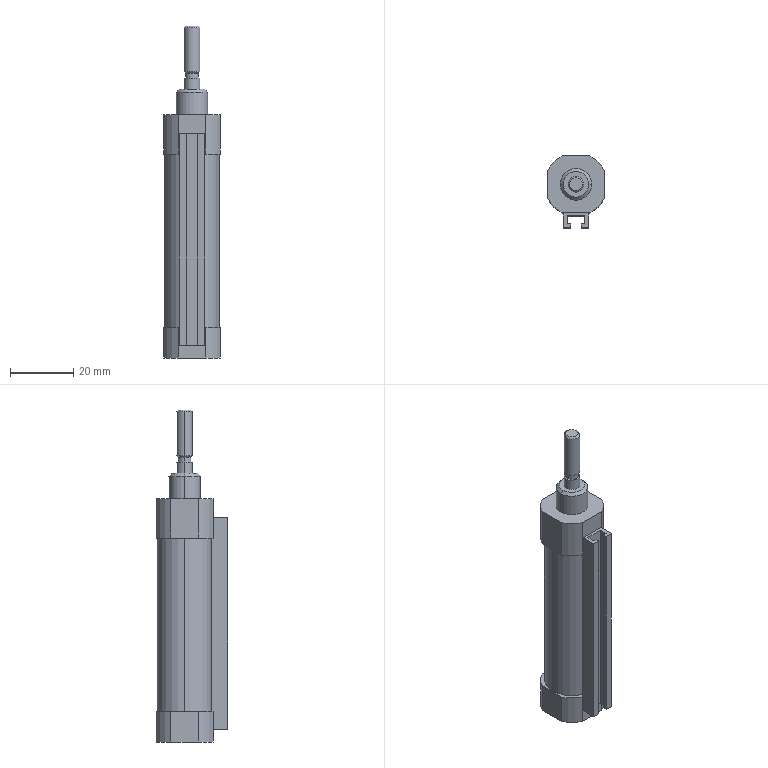Part | STEP file | CDJ2B16-30-B | 1 solid | 65 faces | box 18 x 22.7 x 105 mm | volume 21828 mm3 | plane 32 | cylinder 23 | cone 10 | commonest cylinder face diameters 20 x8 4.13 x4 5 x4 17.4 x3 4.02 x2 10 x2